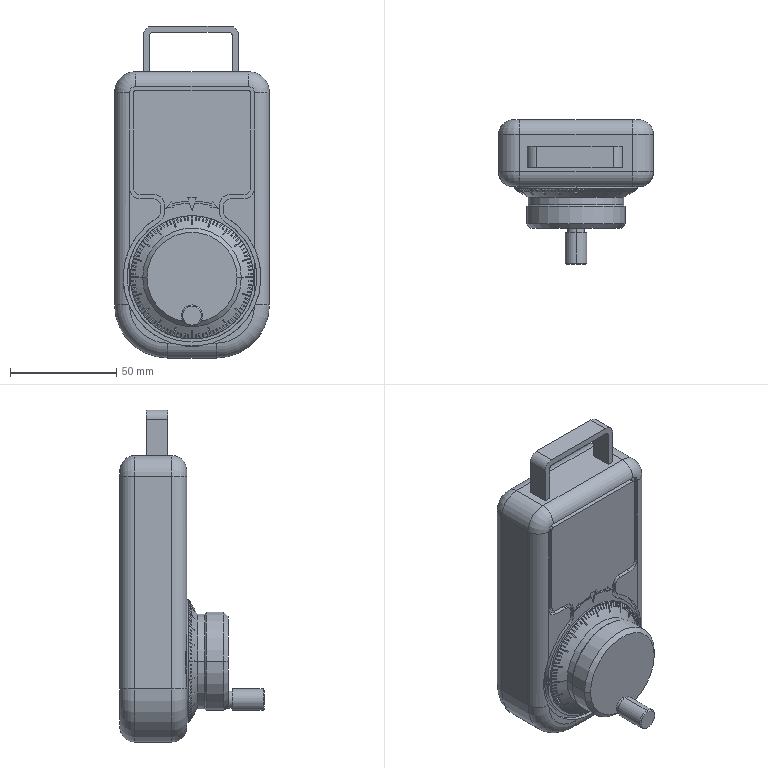Part | NX | features solid 2 | 1 solid | 516 faces | box 73 x 68 x 156.5 mm | volume 329747 mm3 | plane 450 | cylinder 50 | cone 8 | torus 8 | commonest cylinder face diameters 14 x10 6 x8 10 x8 2 x2 3 x2 8 x2